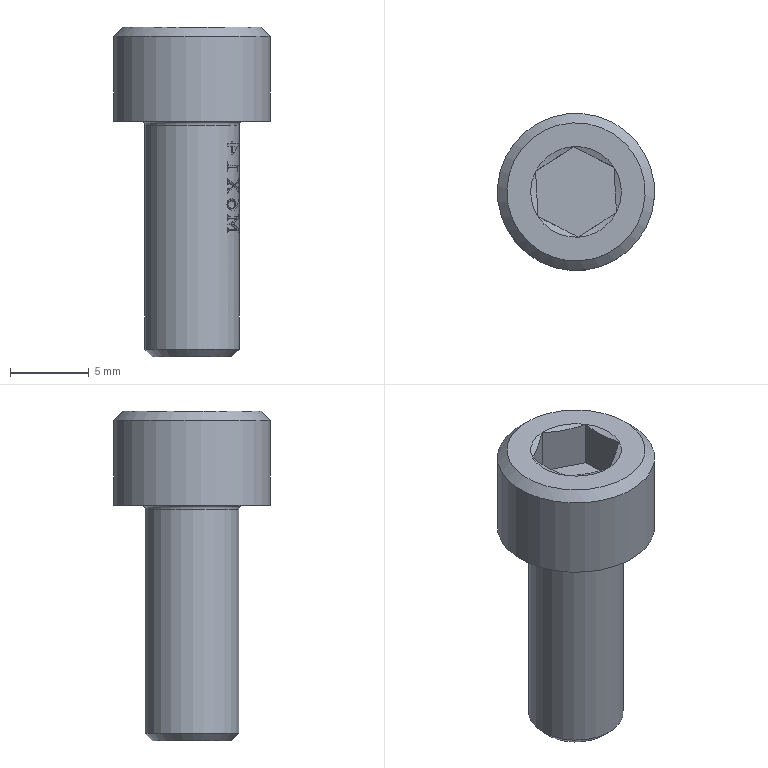Part | STEP file | solid 172 | 1 solid | 108 faces | box 10 x 10 x 21 mm | volume 822.37 mm3 | plane 67 | other 25 | cylinder 7 | sphere 6 | cone 2 | torus 1 | commonest cylinder face diameters 6 x6 10 x1